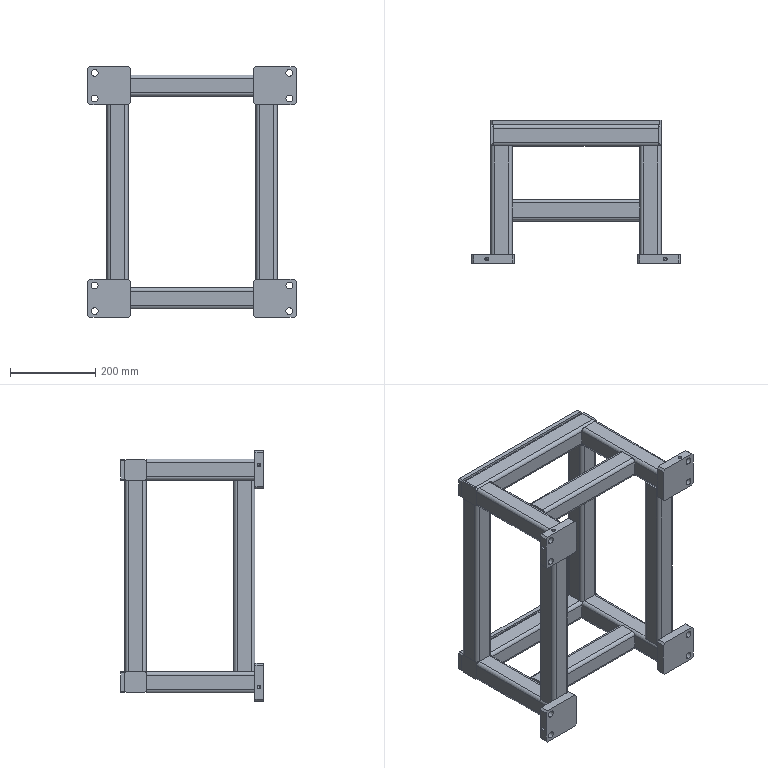Part | SolidWorks | features HoleWzd 6 | 22 solids | 400 faces | box 490 x 336 x 590 mm | volume 4704318 mm3 | plane 220 | cylinder 152 | cone 28 | commonest cylinder face diameters 16 x64 6 x48 6.8 x24 8.5 x16